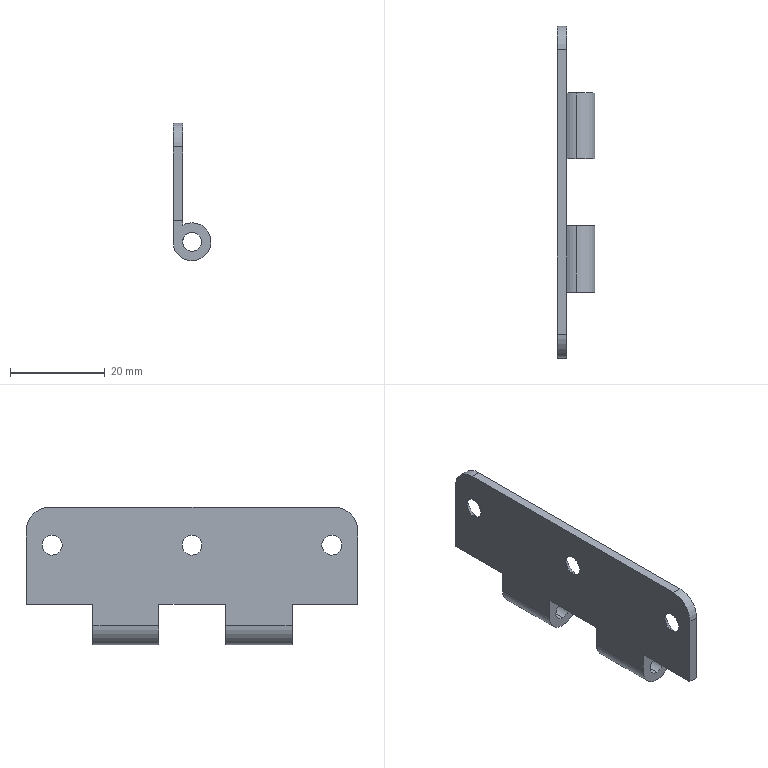Part | SolidWorks | features BaseBody 1 | 1 solid | 36 faces | box 8 x 70 x 29 mm | volume 3838 mm3 | cylinder 18 | plane 12 | cone 6 | commonest cylinder face diameters 4.2 x6 8 x6 4 x4 10 x2